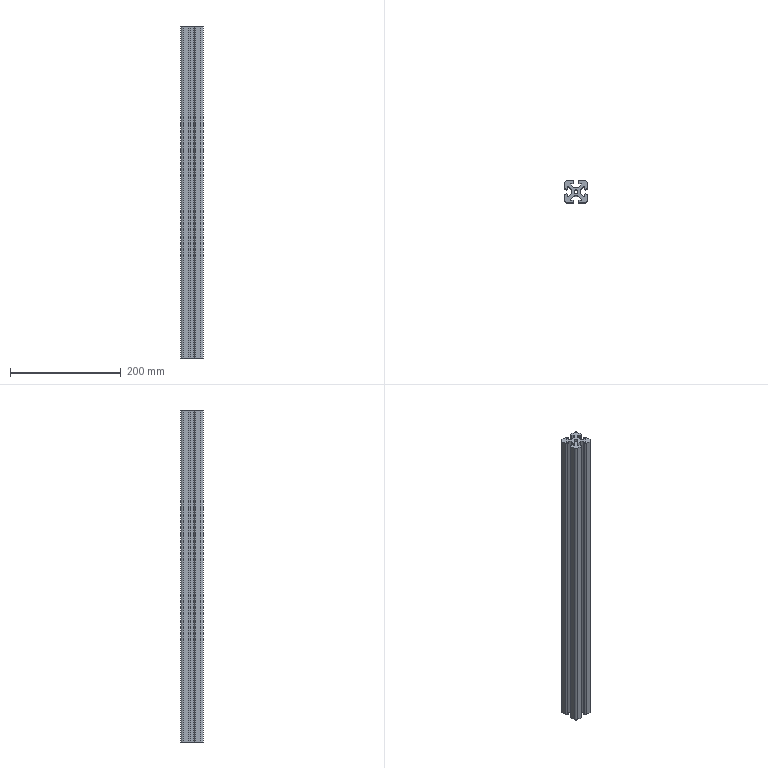Part | SolidWorks | features Extrusion 1 | 1 solid | 78 faces | box 40 x 40 x 600 mm | volume 570398 mm3 | cylinder 48 | plane 30 | commonest cylinder face diameters 2 x26 4 x8 49.184 x8 8 x4 6.8 x2